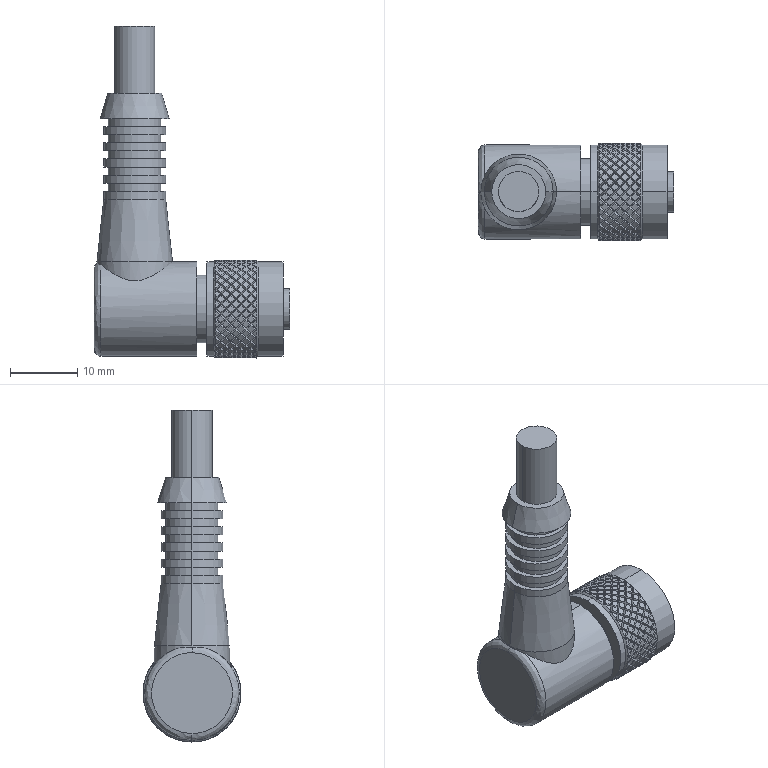Part | SolidWorks | features BaseBody 1 | 1 solid | 1656 faces | box 29 x 14.5 x 49.25 mm | volume 6305 mm3 | spline 1202 | cylinder 309 | plane 137 | cone 8 | commonest cylinder face diameters 14.5 x275 7.8 x10 9.2 x10 14 x6 6 x4 10 x2